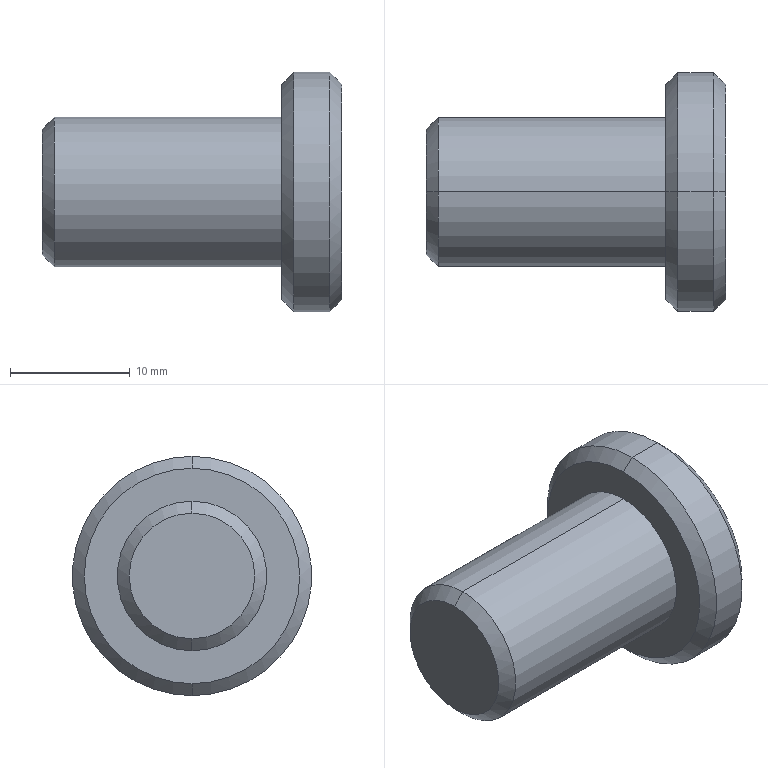Part | SolidWorks | features Chamfer 1, Revolution 1 | 1 solid | 13 faces | box 25 x 20 x 20 mm | volume 3946 mm3 | cone 6 | cylinder 4 | plane 3 | commonest cylinder face diameters 12.5 x2 20 x2
STEP:
#1=CARTESIAN_POINT('',(236.937,-170.509,5.25));
#2=VERTEX_POINT('',#1);
#3=CARTESIAN_POINT('',(236.937,-170.509,-5.25));
#4=VERTEX_POINT('',#3);
#5=CARTESIAN_POINT('',(236.937,-170.509,0.));
#6=DIRECTION('',(-1.,0.,0.));
#7=DIRECTION('',(0.,0.,-1.));
#8=AXIS2_PLACEMENT_3D('',#5,#6,#7);
#9=CIRCLE('',#8,5.25);
#10=EDGE_CURVE('',#2,#4,#9,.T.);
#11=ORIENTED_EDGE('',*,*,#10,.F.);
#12=CARTESIAN_POINT('',(237.937,-170.509,6.25));
#13=VERTEX_POINT('',#12);
#14=CARTESIAN_POINT('',(236.937,-170.509,5.25));
#15=DIRECTION('',(0.7071,0.,0.7071));
#16=VECTOR('',#15,1000.);
#17=LINE('',#14,#16);
#18=EDGE_CURVE('',#2,#13,#17,.T.);
#19=ORIENTED_EDGE('',*,*,#18,.T.);
#20=CARTESIAN_POINT('',(237.937,-170.509,-6.25));
#21=VERTEX_POINT('',#20);
#22=CARTESIAN_POINT('',(237.937,-170.509,0.));
#23=DIRECTION('',(1.,0.,0.));
#24=DIRECTION('',(0.,0.,-1.));
#25=AXIS2_PLACEMENT_3D('',#22,#23,#24);
#26=CIRCLE('',#25,6.25);
#27=EDGE_CURVE('',#21,#13,#26,.T.);
#28=ORIENTED_EDGE('',*,*,#27,.F.);
#29=CARTESIAN_POINT('',(236.937,-170.509,-5.25));
#30=DIRECTION('',(0.7071,0.,-0.7071));
#31=VECTOR('',#30,1000.);
#32=LINE('',#29,#31);
#33=EDGE_CURVE('',#4,#21,#32,.T.);
#34=ORIENTED_EDGE('',*,*,#33,.F.);
#35=EDGE_LOOP('',(#11,#19,#28,#34));
#36=FACE_OUTER_BOUND('',#35,.T.);
#37=CARTESIAN_POINT('',(236.937,-170.509,0.));
#38=DIRECTION('',(1.,0.,0.));
#39=DIRECTION('',(0.,0.,-1.));
#40=AXIS2_PLACEMENT_3D('',#37,#38,#39);
#41=CONICAL_SURFACE('',#40,5.25,0.7854);
#42=ADVANCED_FACE('',(#36),#41,.T.);
#43=CARTESIAN_POINT('',(256.937,-170.509,9.));
#44=VERTEX_POINT('',#43);
#45=CARTESIAN_POINT('',(256.937,-170.509,-9.));
#46=VERTEX_POINT('',#45);
#47=CARTESIAN_POINT('',(256.937,-170.509,0.));
#48=DIRECTION('',(-1.,0.,0.));
#49=DIRECTION('',(0.,0.,-1.));
#50=AXIS2_PLACEMENT_3D('',#47,#48,#49);
#51=CIRCLE('',#50,9.);
#52=EDGE_CURVE('',#44,#46,#51,.T.);
#53=ORIENTED_EDGE('',*,*,#52,.F.);
#54=CARTESIAN_POINT('',(257.937,-170.509,10.));
#55=VERTEX_POINT('',#54);
#56=CARTESIAN_POINT('',(256.937,-170.509,9.));
#57=DIRECTION('',(0.7071,0.,0.7071));
#58=VECTOR('',#57,1000.);
#59=LINE('',#56,#58);
#60=EDGE_CURVE('',#44,#55,#59,.T.);
#61=ORIENTED_EDGE('',*,*,#60,.T.);
#62=CARTESIAN_POINT('',(257.937,-170.509,-10.));
#63=VERTEX_POINT('',#62);
#64=CARTESIAN_POINT('',(257.937,-170.509,0.));
#65=DIRECTION('',(1.,0.,0.));
#66=DIRECTION('',(0.,0.,-1.));
#67=AXIS2_PLACEMENT_3D('',#64,#65,#66);
#68=CIRCLE('',#67,10.);
#69=EDGE_CURVE('',#63,#55,#68,.T.);
#70=ORIENTED_EDGE('',*,*,#69,.F.);
#71=CARTESIAN_POINT('',(256.937,-170.509,-9.));
#72=DIRECTION('',(0.7071,0.,-0.7071));
#73=VECTOR('',#72,1000.);
#74=LINE('',#71,#73);
#75=EDGE_CURVE('',#46,#63,#74,.T.);
#76=ORIENTED_EDGE('',*,*,#75,.F.);
#77=EDGE_LOOP('',(#53,#61,#70,#76));
#78=FACE_OUTER_BOUND('',#77,.T.);
#79=CARTESIAN_POINT('',(256.937,-170.509,0.));
#80=DIRECTION('',(1.,0.,0.));
#81=DIRECTION('',(0.,0.,-1.));
#82=AXIS2_PLACEMENT_3D('',#79,#80,#81);
#83=CONICAL_SURFACE('',#82,9.,0.7854);
#84=ADVANCED_FACE('',(#78),#83,.T.);
#85=CARTESIAN_POINT('',(261.937,-170.509,-9.));
#86=VERTEX_POINT('',#85);
#87=CARTESIAN_POINT('',(261.937,-170.509,9.));
#88=VERTEX_POINT('',#87);
#89=CARTESIAN_POINT('',(261.937,-170.509,0.));
#90=DIRECTION('',(1.,0.,0.));
#91=DIRECTION('',(0.,0.,1.));
#92=AXIS2_PLACEMENT_3D('',#89,#90,#91);
#93=CIRCLE('',#92,9.);
#94=EDGE_CURVE('',#86,#88,#93,.T.);
#95=ORIENTED_EDGE('',*,*,#94,.F.);
#96=CARTESIAN_POINT('',(260.937,-170.509,-10.));
#97=VERTEX_POINT('',#96);
#98=CARTESIAN_POINT('',(260.937,-170.509,-10.));
#99=DIRECTION('',(-0.7071,0.,-0.7071));
#100=VECTOR('',#99,1000.);
#101=LINE('',#98,#100);
#102=EDGE_CURVE('',#86,#97,#101,.T.);
#103=ORIENTED_EDGE('',*,*,#102,.T.);
#104=CARTESIAN_POINT('',(260.937,-170.509,10.));
#105=VERTEX_POINT('',#104);
#106=CARTESIAN_POINT('',(260.937,-170.509,0.));
#107=DIRECTION('',(-1.,0.,0.));
#108=DIRECTION('',(0.,0.,1.));
#109=AXIS2_PLACEMENT_3D('',#106,#107,#108);
#110=CIRCLE('',#109,10.);
#111=EDGE_CURVE('',#105,#97,#110,.T.);
#112=ORIENTED_EDGE('',*,*,#111,.F.);
#113=CARTESIAN_POINT('',(260.937,-170.509,10.));
#114=DIRECTION('',(-0.7071,0.,0.7071));
#115=VECTOR('',#114,1000.);
#116=LINE('',#113,#115);
#117=EDGE_CURVE('',#88,#105,#116,.T.);
#118=ORIENTED_EDGE('',*,*,#117,.F.);
#119=EDGE_LOOP('',(#95,#103,#112,#118));
#120=FACE_OUTER_BOUND('',#119,.T.);
#121=CARTESIAN_POINT('',(260.937,-170.509,0.));
#122=DIRECTION('',(-1.,0.,0.));
#123=DIRECTION('',(0.,0.,1.));
#124=AXIS2_PLACEMENT_3D('',#121,#122,#123);
#125=CONICAL_SURFACE('',#124,10.,0.7854);
#126=ADVANCED_FACE('',(#120),#125,.T.);
#127=ORIENTED_EDGE('',*,*,#111,.T.);
#128=CARTESIAN_POINT('',(232.937,-170.509,-10.));
#129=DIRECTION('',(-1.,0.,0.));
#130=VECTOR('',#129,1000.);
#131=LINE('',#128,#130);
#132=EDGE_CURVE('',#97,#63,#131,.T.);
#133=ORIENTED_EDGE('',*,*,#132,.T.);
#134=ORIENTED_EDGE('',*,*,#69,.T.);
#135=CARTESIAN_POINT('',(232.937,-170.509,10.));
#136=DIRECTION('',(-1.,0.,0.));
#137=VECTOR('',#136,1000.);
#138=LINE('',#135,#137);
#139=EDGE_CURVE('',#105,#55,#138,.T.);
#140=ORIENTED_EDGE('',*,*,#139,.F.);
#141=EDGE_LOOP('',(#127,#133,#134,#140));
#142=FACE_OUTER_BOUND('',#141,.T.);
#143=CARTESIAN_POINT('',(232.937,-170.509,0.));
#144=DIRECTION('',(-1.,0.,0.));
#145=DIRECTION('',(0.,0.,1.));
#146=AXIS2_PLACEMENT_3D('',#143,#144,#145);
#147=CYLINDRICAL_SURFACE('',#146,10.);
#148=ADVANCED_FACE('',(#142),#147,.T.);
#149=CARTESIAN_POINT('',(256.937,-170.509,6.25));
#150=VERTEX_POINT('',#149);
#151=CARTESIAN_POINT('',(256.937,-170.509,-6.25));
#152=VERTEX_POINT('',#151);
#153=CARTESIAN_POINT('',(256.937,-170.509,0.));
#154=DIRECTION('',(-1.,0.,0.));
#155=DIRECTION('',(0.,0.,1.));
#156=AXIS2_PLACEMENT_3D('',#153,#154,#155);
#157=CIRCLE('',#156,6.25);
#158=EDGE_CURVE('',#150,#152,#157,.T.);
#159=ORIENTED_EDGE('',*,*,#158,.T.);
#160=CARTESIAN_POINT('',(232.937,-170.509,-6.25));
#161=DIRECTION('',(-1.,0.,0.));
#162=VECTOR('',#161,1000.);
#163=LINE('',#160,#162);
#164=EDGE_CURVE('',#152,#21,#163,.T.);
#165=ORIENTED_EDGE('',*,*,#164,.T.);
#166=ORIENTED_EDGE('',*,*,#27,.T.);
#167=CARTESIAN_POINT('',(232.937,-170.509,6.25));
#168=DIRECTION('',(-1.,0.,0.));
#169=VECTOR('',#168,1000.);
#170=LINE('',#167,#169);
#171=EDGE_CURVE('',#150,#13,#170,.T.);
#172=ORIENTED_EDGE('',*,*,#171,.F.);
#173=EDGE_LOOP('',(#159,#165,#166,#172));
#174=FACE_OUTER_BOUND('',#173,.T.);
#175=CARTESIAN_POINT('',(232.937,-170.509,0.));
#176=DIRECTION('',(-1.,0.,0.));
#177=DIRECTION('',(0.,0.,1.));
#178=AXIS2_PLACEMENT_3D('',#175,#176,#177);
#179=CYLINDRICAL_SURFACE('',#178,6.25);
#180=ADVANCED_FACE('',(#174),#179,.T.);
#181=CARTESIAN_POINT('',(236.937,-170.509,0.));
#182=DIRECTION('',(-1.,0.,0.));
#183=DIRECTION('',(0.,0.,-1.));
#184=AXIS2_PLACEMENT_3D('',#181,#182,#183);
#185=CIRCLE('',#184,5.25);
#186=EDGE_CURVE('',#4,#2,#185,.T.);
#187=ORIENTED_EDGE('',*,*,#186,.T.);
#188=ORIENTED_EDGE('',*,*,#10,.T.);
#189=EDGE_LOOP('',(#187,#188));
#190=FACE_OUTER_BOUND('',#189,.T.);
#191=CARTESIAN_POINT('',(236.937,-170.509,0.));
#192=DIRECTION('',(1.,0.,0.));
#193=DIRECTION('',(0.,0.,-1.));
#194=AXIS2_PLACEMENT_3D('',#191,#192,#193);
#195=PLANE('',#194);
#196=ADVANCED_FACE('',(#190),#195,.F.);
#197=ORIENTED_EDGE('',*,*,#164,.F.);
#198=CARTESIAN_POINT('',(256.937,-170.509,0.));
#199=DIRECTION('',(-1.,0.,0.));
#200=DIRECTION('',(0.,0.,1.));
#201=AXIS2_PLACEMENT_3D('',#198,#199,#200);
#202=CIRCLE('',#201,6.25);
#203=EDGE_CURVE('',#152,#150,#202,.T.);
#204=ORIENTED_EDGE('',*,*,#203,.T.);
#205=ORIENTED_EDGE('',*,*,#171,.T.);
#206=CARTESIAN_POINT('',(237.937,-170.509,0.));
#207=DIRECTION('',(1.,0.,0.));
#208=DIRECTION('',(0.,0.,-1.));
#209=AXIS2_PLACEMENT_3D('',#206,#207,#208);
#210=CIRCLE('',#209,6.25);
#211=EDGE_CURVE('',#13,#21,#210,.T.);
#212=ORIENTED_EDGE('',*,*,#211,.T.);
#213=EDGE_LOOP('',(#197,#204,#205,#212));
#214=FACE_OUTER_BOUND('',#213,.T.);
#215=CARTESIAN_POINT('',(232.937,-170.509,0.));
#216=DIRECTION('',(-1.,0.,0.));
#217=DIRECTION('',(0.,0.,1.));
#218=AXIS2_PLACEMENT_3D('',#215,#216,#217);
#219=CYLINDRICAL_SURFACE('',#218,6.25);
#220=ADVANCED_FACE('',(#214),#219,.T.);
#221=CARTESIAN_POINT('',(256.937,-170.509,0.));
#222=DIRECTION('',(-1.,0.,0.));
#223=DIRECTION('',(0.,0.,-1.));
#224=AXIS2_PLACEMENT_3D('',#221,#222,#223);
#225=CIRCLE('',#224,9.);
#226=EDGE_CURVE('',#46,#44,#225,.T.);
#227=ORIENTED_EDGE('',*,*,#226,.T.);
#228=ORIENTED_EDGE('',*,*,#52,.T.);
#229=EDGE_LOOP('',(#227,#228));
#230=FACE_OUTER_BOUND('',#229,.T.);
#231=ORIENTED_EDGE('',*,*,#158,.F.);
#232=ORIENTED_EDGE('',*,*,#203,.F.);
#233=EDGE_LOOP('',(#231,#232));
#234=FACE_BOUND('',#233,.T.);
#235=CARTESIAN_POINT('',(256.937,-164.259,0.));
#236=DIRECTION('',(1.,0.,0.));
#237=DIRECTION('',(0.,0.,-1.));
#238=AXIS2_PLACEMENT_3D('',#235,#236,#237);
#239=PLANE('',#238);
#240=ADVANCED_FACE('',(#230,#234),#239,.F.);
#241=ORIENTED_EDGE('',*,*,#132,.F.);
#242=CARTESIAN_POINT('',(260.937,-170.509,0.));
#243=DIRECTION('',(-1.,0.,0.));
#244=DIRECTION('',(0.,0.,1.));
#245=AXIS2_PLACEMENT_3D('',#242,#243,#244);
#246=CIRCLE('',#245,10.);
#247=EDGE_CURVE('',#97,#105,#246,.T.);
#248=ORIENTED_EDGE('',*,*,#247,.T.);
#249=ORIENTED_EDGE('',*,*,#139,.T.);
#250=CARTESIAN_POINT('',(257.937,-170.509,0.));
#251=DIRECTION('',(1.,0.,0.));
#252=DIRECTION('',(0.,0.,-1.));
#253=AXIS2_PLACEMENT_3D('',#250,#251,#252);
#254=CIRCLE('',#253,10.);
#255=EDGE_CURVE('',#55,#63,#254,.T.);
#256=ORIENTED_EDGE('',*,*,#255,.T.);
#257=EDGE_LOOP('',(#241,#248,#249,#256));
#258=FACE_OUTER_BOUND('',#257,.T.);
#259=CARTESIAN_POINT('',(232.937,-170.509,0.));
#260=DIRECTION('',(-1.,0.,0.));
#261=DIRECTION('',(0.,0.,1.));
#262=AXIS2_PLACEMENT_3D('',#259,#260,#261);
#263=CYLINDRICAL_SURFACE('',#262,10.);
#264=ADVANCED_FACE('',(#258),#263,.T.);
#265=CARTESIAN_POINT('',(261.937,-170.509,0.));
#266=DIRECTION('',(1.,0.,0.));
#267=DIRECTION('',(0.,0.,1.));
#268=AXIS2_PLACEMENT_3D('',#265,#266,#267);
#269=CIRCLE('',#268,9.);
#270=EDGE_CURVE('',#88,#86,#269,.T.);
#271=ORIENTED_EDGE('',*,*,#270,.T.);
#272=ORIENTED_EDGE('',*,*,#94,.T.);
#273=EDGE_LOOP('',(#271,#272));
#274=FACE_OUTER_BOUND('',#273,.T.);
#275=CARTESIAN_POINT('',(261.937,-160.509,0.));
#276=DIRECTION('',(-1.,0.,0.));
#277=DIRECTION('',(0.,0.,1.));
#278=AXIS2_PLACEMENT_3D('',#275,#276,#277);
#279=PLANE('',#278);
#280=ADVANCED_FACE('',(#274),#279,.F.);
#281=ORIENTED_EDGE('',*,*,#102,.F.);
#282=ORIENTED_EDGE('',*,*,#270,.F.);
#283=ORIENTED_EDGE('',*,*,#117,.T.);
#284=ORIENTED_EDGE('',*,*,#247,.F.);
#285=EDGE_LOOP('',(#281,#282,#283,#284));
#286=FACE_OUTER_BOUND('',#285,.T.);
#287=CARTESIAN_POINT('',(260.937,-170.509,0.));
#288=DIRECTION('',(-1.,0.,0.));
#289=DIRECTION('',(0.,0.,1.));
#290=AXIS2_PLACEMENT_3D('',#287,#288,#289);
#291=CONICAL_SURFACE('',#290,10.,0.7854);
#292=ADVANCED_FACE('',(#286),#291,.T.);
#293=ORIENTED_EDGE('',*,*,#60,.F.);
#294=ORIENTED_EDGE('',*,*,#226,.F.);
#295=ORIENTED_EDGE('',*,*,#75,.T.);
#296=ORIENTED_EDGE('',*,*,#255,.F.);
#297=EDGE_LOOP('',(#293,#294,#295,#296));
#298=FACE_OUTER_BOUND('',#297,.T.);
#299=CARTESIAN_POINT('',(256.937,-170.509,0.));
#300=DIRECTION('',(1.,0.,0.));
#301=DIRECTION('',(0.,0.,-1.));
#302=AXIS2_PLACEMENT_3D('',#299,#300,#301);
#303=CONICAL_SURFACE('',#302,9.,0.7854);
#304=ADVANCED_FACE('',(#298),#303,.T.);
#305=ORIENTED_EDGE('',*,*,#18,.F.);
#306=ORIENTED_EDGE('',*,*,#186,.F.);
#307=ORIENTED_EDGE('',*,*,#33,.T.);
#308=ORIENTED_EDGE('',*,*,#211,.F.);
#309=EDGE_LOOP('',(#305,#306,#307,#308));
#310=FACE_OUTER_BOUND('',#309,.T.);
#311=CARTESIAN_POINT('',(236.937,-170.509,0.));
#312=DIRECTION('',(1.,0.,0.));
#313=DIRECTION('',(0.,0.,-1.));
#314=AXIS2_PLACEMENT_3D('',#311,#312,#313);
#315=CONICAL_SURFACE('',#314,5.25,0.7854);
#316=ADVANCED_FACE('',(#310),#315,.T.);
#317=CLOSED_SHELL('',(#42,#84,#126,#148,#180,#196,#220,#240,#264,#280,#292,#304,#316));
#318=MANIFOLD_SOLID_BREP('',#317);
#319=CARTESIAN_POINT('',(0.,0.,0.));
#320=DIRECTION('',(0.,0.,1.));
#321=DIRECTION('',(1.,0.,0.));
#322=AXIS2_PLACEMENT_3D('',#319,#320,#321);
#323=(LENGTH_UNIT()NAMED_UNIT(*)SI_UNIT(.MILLI.,.METRE.));
#324=UNCERTAINTY_MEASURE_WITH_UNIT(LENGTH_MEASURE(0.00001),#323,'','');
#325=(NAMED_UNIT(*)PLANE_ANGLE_UNIT()SI_UNIT($,.RADIAN.));
#326=(NAMED_UNIT(*)SI_UNIT($,.STERADIAN.)SOLID_ANGLE_UNIT());
#327=(GEOMETRIC_REPRESENTATION_CONTEXT(3)GLOBAL_UNCERTAINTY_ASSIGNED_CONTEXT((#324))GLOBAL_UNIT_ASSIGNED_CONTEXT((#323,#325,#326))REPRESENTATION_CONTEXT('',''));
#328=ADVANCED_BREP_SHAPE_REPRESENTATION('',(#318,#322),#327);